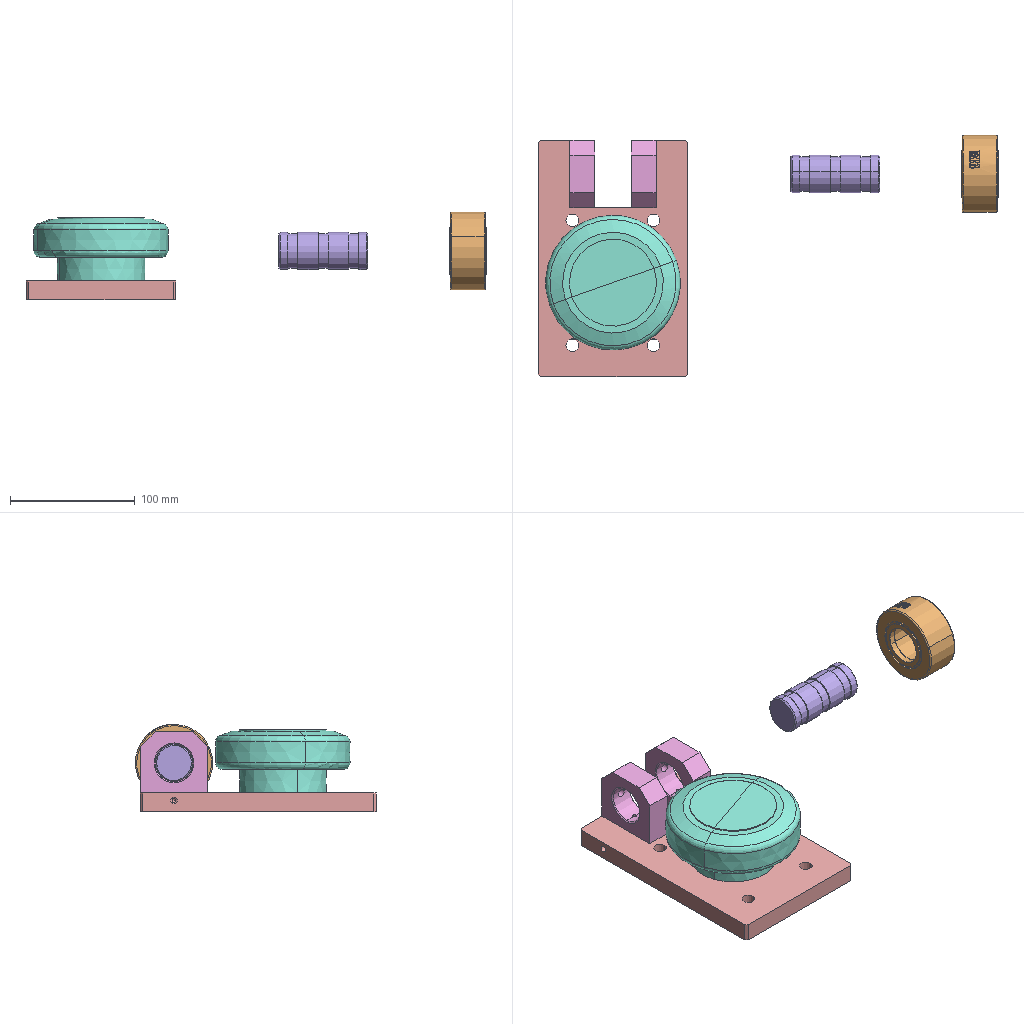Assembly | SolidWorks | 6 different items | 7 placed | box 368 x 193 x 70 mm
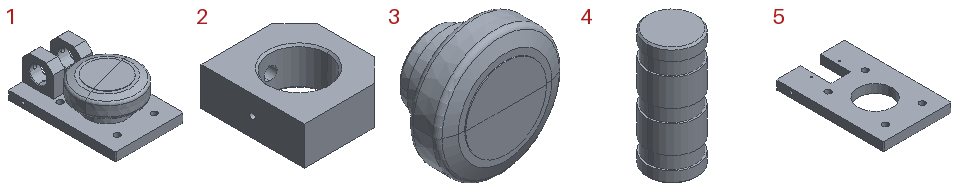Parts list (item | name | quantity | size | volume | features):
1 | (subassembly) | x1 | 120 x 189 x 65.476 mm | 714505 mm3 | features CompositeCurve 2
2 | - | x2 | 49 x 54 x 20 mm | 35303 mm3 | features 3DProfileFeature 2, HoleWzd 2, Chamfer 1, Extrusion 1, ICE 1
3 | - | x1 | 107.698 x 64.478 x 107.698 mm | 380558 mm3 | features Revolution 1
4 | - | x1 | 30 x 30 x 71 mm | 47169 mm3 | features HoleWzd 3, 3DProfileFeature 2, Chamfer 1, Extrusion 1, ICE 1, RevCut 1
5 | - | x1 | 120 x 189 x 15 mm | 263341 mm3 | features 3DProfileFeature 6, HoleWzd 6, ICE 2, Extrusion 1
6 | NUTR30.stp | x1 | - | - | -
Mates (type | each side: item.copy, entity, surface, feature):
Concentric | 5.1 face cylinder Size mm dowel hole 3 | 2.1 face cylinder Size mm dowel hole 1
Coincident | 5.1 face plane Boss-Extrude1 | 2.1 face plane Boss-Extrude1 | 2 times
Concentric | 5.1 face cylinder Size mm dowel hole 3 | 2.2 face cylinder Size mm dowel hole 1
Coincident | 5.1 face plane Boss-Extrude1 | 2.2 face plane Boss-Extrude1 | 2 times
Concentric | 5.1 face cylinder Cut-Extrude8 | 3.1 face cone Revolve1
DistanceDim | 4.1 face plane Boss-Extrude1 | 2.2 face plane Boss-Extrude1
Concentric | 2.2 face cylinder Cut-Extrude1 | 4.1 face cylinder Boss-Extrude1
Coincident | 5.1 face plane Boss-Extrude1 | 3.1 edge